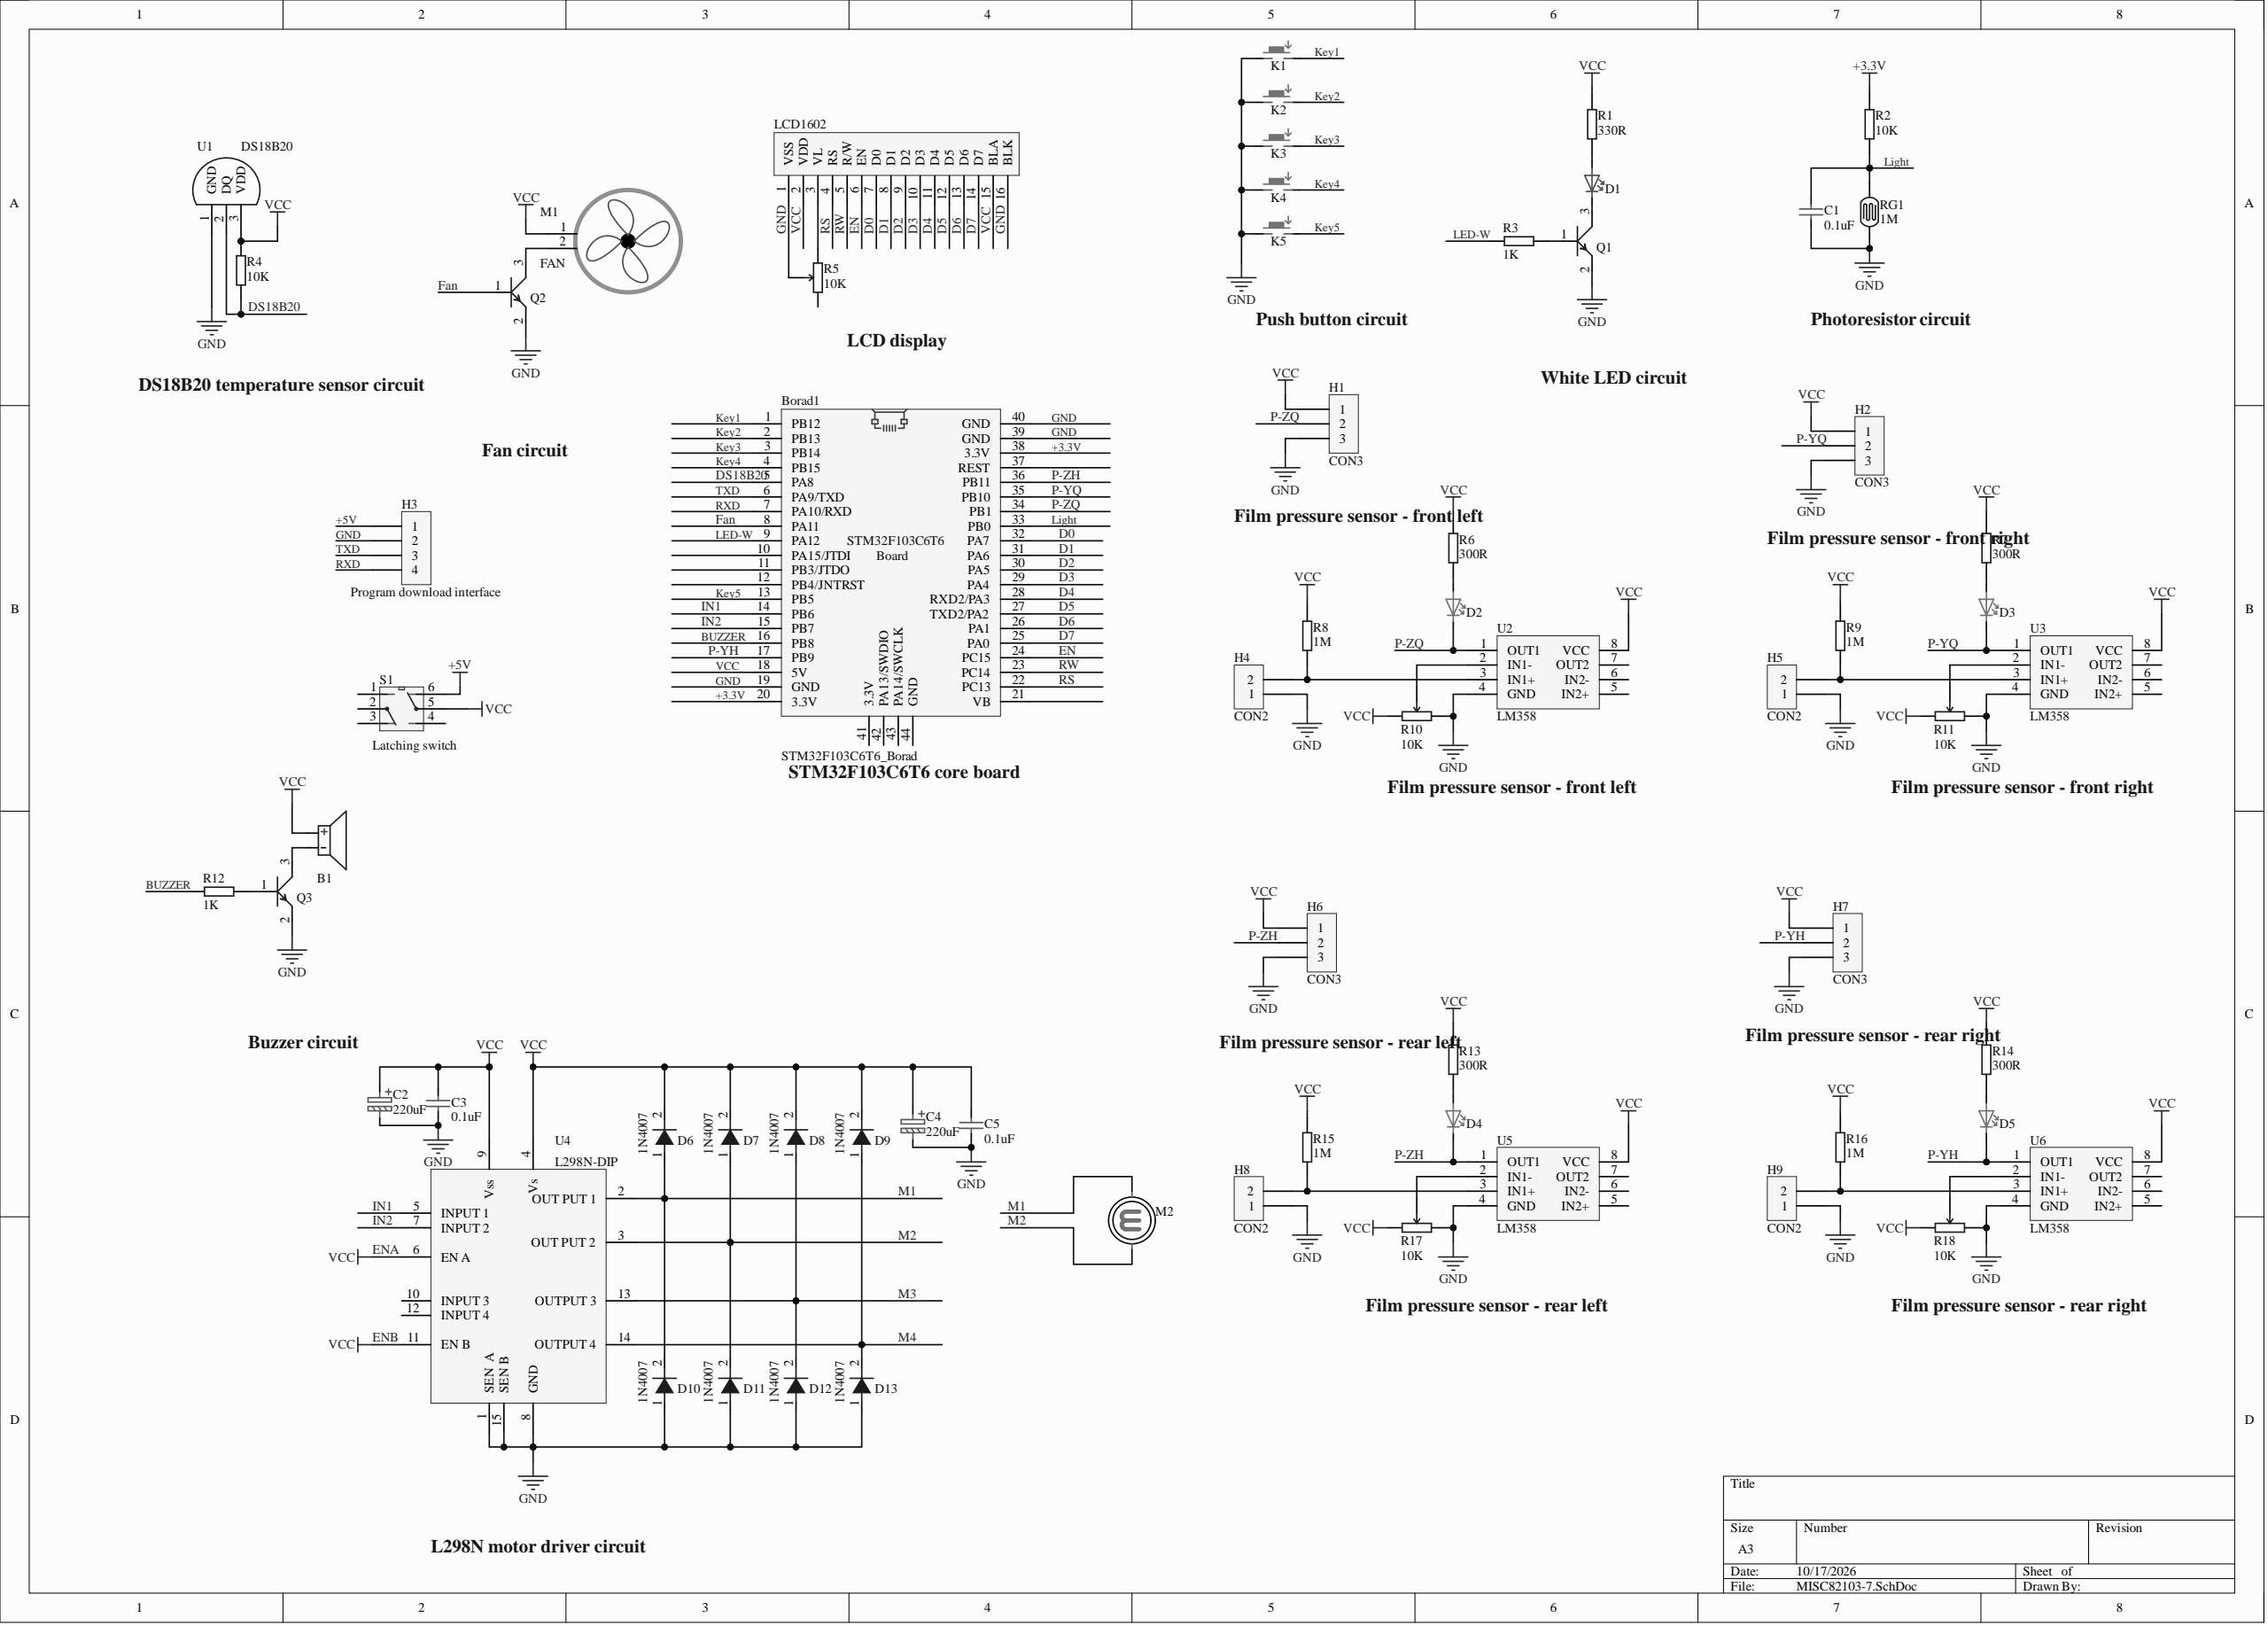Circuit board | Altium Designer | 66 parts | 56 nets
Bill of materials:
Comment,Description,Designator,Footprint,LibRef,Quantity
"Buzzer","Buzzer","B1","BUZZER","Buzzer","1"
"STM32F103C6T6_Borad","Core board (purchased online)","Borad1","STM32F103C8T6_买的","STM32F103C6T6_Borad","1"
"0.1uF","Non-polar capacitor","C1, C3, C5","CAP - 2.54mm","CAP","3"
"220uF","Polar capacitor","C2, C4","CAPe - 3.5MM","CAP-E","2"
"LED","LED","D1, D2, D3, D4, D5","LED-3MM","LED-RED, LED-GREEN","5"
"1N4007","Rectifier diode / single-direction diode","D6, D7, D8, D9, D10, D11, D12, D13","DIODE - 15.24mm","Diode","8"
"CON3","Pin header / terminal block / connector","H1, H2, H6, H7","CON3","CON3","4"
"Program download interface","Pin header / terminal block / connector","H3","CON4","CON4","1"
"CON2","Pin header / terminal block / connector","H4, H5, H8, H9","CON2","CON2","4"
"Key","Push button","K1, K2, K3, K4, K5","Buttom","Key","5"
"LCD1602","","LCD1","LCD1602","LCD1602","1"
"FAN","Small fan","M1","CON2","FAN","1"
"MOTTOR","DC motor","M2","CON2","MOTTOR","1"
"NPN","NPN transistor","Q1, Q2, Q3","NPN & PNP","NPN","3"
"330R","Resistor","R1","Resistor-7.62mm","Res","1"
"10K","Resistor","R2, R4","Resistor-7.62mm","Res","2"
"1K","Resistor","R3, R12","Resistor-7.62mm","Res","2"
"10K","Adjustable resistor","R5, R10, R11, R17, R18","Res_Variable-DIP","Res_Variable","5"
"300R","Resistor","R6, R7, R13, R14","Resistor-7.62mm","Res","4"
"1M","Resistor","R8, R9, R15, R16","Resistor-7.62mm","Res","4"
"1M","Photoresistor","RG1","RG","RG","1"
"Latching switch","8*8 power switch / latching switch","S1","Switch","Switch","1"
"DS18B20","Temperature sensor","U1","DS18B20","DS18B20","1"
"LM358","Dual operational amplifier","U2, U3, U5, U6","DIP8","LM358","4"
"L298N-DIP","Dual H-bridge driver IC","U4","L298N","L298N-DIP","1"
Netlist (Protel format):
[
B1
BUZZER
Buzzer



]
[
Borad1
STM32F103C8T6_买的
STM32F103C6T6_Borad



]
[
C1
CAP - 2.54mm
0.1uF



]
[
C2
CAPe - 3.5MM
220uF



]
[
C3
CAP - 2.54mm
0.1uF



]
[
C4
CAPe - 3.5MM
220uF



]
[
C5
CAP - 2.54mm
0.1uF



]
[
D1
LED-3MM
LED



]
[
D2
LED-3MM
LED



]
[
D3
LED-3MM
LED



]
[
D4
LED-3MM
LED



]
[
D5
LED-3MM
LED



]
[
D6
DIODE - 15.24mm
1N4007



]
[
D7
DIODE - 15.24mm
1N4007



]
[
D8
DIODE - 15.24mm
1N4007



]
[
D9
DIODE - 15.24mm
1N4007



]
[
D10
DIODE - 15.24mm
1N4007



]
[
D11
DIODE - 15.24mm
1N4007



]
[
D12
DIODE - 15.24mm
1N4007



]
[
D13
DIODE - 15.24mm
1N4007



]
[
H1
CON3
CON3



]
[
H2
CON3
CON3



]
[
H3
CON4
Program download interface



]
[
H4
CON2
CON2



]
[
H5
CON2
CON2



]
[
H6
CON3
CON3



]
[
H7
CON3
CON3



]
[
H8
CON2
CON2



]
[
H9
CON2
CON2



]
[
K1
Buttom
Key



]
[
K2
Buttom
Key



]
[
K3
Buttom
Key



]
[
K4
Buttom
Key



]
[
K5
Buttom
Key



]
[
LCD1
LCD1602
LCD1602



]
[
M1
CON2
FAN



]
[
M2
CON2
MOTTOR



]
[
Q1
NPN & PNP
NPN



]
[
Q2
NPN & PNP
NPN



]
[
Q3
NPN & PNP
NPN



]
[
R1
Resistor-7.62mm
330R



]
[
R2
Resistor-7.62mm
10K



]
[
R3
Resistor-7.62mm
1K



]
[
R4
Resistor-7.62mm
10K



]
[
R5
Res_Variable-DIP
10K



]
[
R6
Resistor-7.62mm
300R



]
[
R7
Resistor-7.62mm
300R



]
[
R8
Resistor-7.62mm
1M



]
[
R9
Resistor-7.62mm
1M



]
[
R10
Res_Variable-DIP
10K



]
[
R11
Res_Variable-DIP
10K



]
[
R12
Resistor-7.62mm
1K



]
[
R13
Resistor-7.62mm
300R



]
[
R14
Resistor-7.62mm
300R



]
[
R15
Resistor-7.62mm
1M



]
[
R16
Resistor-7.62mm
1M



]
[
R17
Res_Variable-DIP
10K



]
[
R18
Res_Variable-DIP
10K



]
[
RG1
RG
1M



]
[
S1
Switch
Latching switch



]
[
U1
DS18B20
DS18B20



]
[
U2
DIP8
LM358



]
[
U3
DIP8
LM358



]
[
U4
L298N
L298N-DIP



]
[
U5
DIP8
LM358



]
[
U6
DIP8
LM358



]
(
TXD
Borad1-6
H3-3
)
(
RXD
Borad1-7
H3-4
)
(
RW
Borad1-23
LCD1-5
)
(
RS
Borad1-22
LCD1-4
)
(
P-ZQ
Borad1-34
D2-1
H1-2
U2-1
)
(
P-ZH
Borad1-36
D4-1
H6-2
U5-1
)
(
P-YQ
Borad1-35
D3-1
H2-2
U3-1
)
(
P-YH
Borad1-17
D5-1
H7-2
U6-1
)
(
NetR18_2
R18-2
U6-2
)
(
NetR17_2
R17-2
U5-2
)
(
NetR11_2
R11-2
U3-2
)
(
NetR10_2
R10-2
U2-2
)
(
NetQ3_1
Q3-1
R12-2
)
(
NetQ1_1
Q1-1
R3-1
)
(
NetM1_2
M1-2
Q2-3
)
(
NetLCD1_3
LCD1-3
R5-1
)
(
NetH9_2
H9-2
R16-1
U6-3
)
(
NetH8_2
H8-2
R15-1
U5-3
)
(
NetH5_2
H5-2
R9-1
U3-3
)
(
NetH4_2
H4-2
R8-1
U2-3
)
(
NetD5_2
D5-2
R14-1
)
(
NetD4_2
D4-2
R13-1
)
(
NetD3_2
D3-2
R7-1
)
(
NetD2_2
D2-2
R6-1
)
(
NetD1_2
D1-2
R1-1
)
(
NetD1_1
D1-1
Q1-3
)
(
NetB1_2
B1-2
Q3-3
)
(
M4
D9-1
D13-2
U4-14
)
(
M3
D8-1
D12-2
U4-13
)
(
M2
D7-1
D11-2
M2-1
U4-3
)
(
M1
D6-1
D10-2
M2-2
U4-2
)
(
Light
Borad1-33
C1-2
R2-1
RG1-2
)
(
LED-W
Borad1-9
R3-2
)
(
Key5
Borad1-13
K5-2
)
(
Key4
Borad1-4
K4-2
)
(
Key3
Borad1-3
K3-2
)
(
Key2
Borad1-2
K2-2
)
(
Key1
Borad1-1
K1-2
)
(
IN2
Borad1-15
U4-7
)
(
IN1
Borad1-14
U4-5
)
(
GND
Borad1-19
Borad1-39
Borad1-40
C1-1
C2-2
C3-1
C4-2
C5-1
D10-1
D11-1
D12-1
D13-1
H1-3
H2-3
H3-2
H4-1
H5-1
H6-3
H7-3
H8-1
H9-1
K1-1
K2-1
K3-1
K4-1
K5-1
LCD1-1
LCD1-16
Q1-2
Q2-2
Q3-2
R5-2
R10-1
R11-1
R17-1
R18-1
RG1-1
U1-1
U2-4
U3-4
U4-1
U4-8
U4-15
U5-4
U6-4
)
(
Fan
Borad1-8
Q2-1
)
(
ENA
B1-1
Borad1-18
C2-1
C3-2
C4-1
C5-2
D6-2
D7-2
D8-2
D9-2
H1-1
H2-1
H6-1
H7-1
LCD1-2
LCD1-15
M1-1
R1-2
R4-1
R6-2
R7-2
R8-2
R9-2
R10-3
R11-3
R13-2
R14-2
R15-2
R16-2
R17-3
R18-3
S1-5
U1-3
U2-8
U3-8
U4-4
U4-6
U4-9
U4-11
U5-8
U6-8
)
(
EN
Borad1-24
LCD1-6
)
(
DS18B20
Borad1-5
R4-2
U1-2
)
(
D7
Borad1-25
LCD1-14
)
(
D6
Borad1-26
LCD1-13
)
(
D5
Borad1-27
LCD1-12
)
(
D4
Borad1-28
LCD1-11
)
(
D3
Borad1-29
LCD1-10
)
(
D2
Borad1-30
LCD1-9
)
(
D1
Borad1-31
LCD1-8
)
(
D0
Borad1-32
LCD1-7
)
(
BUZZER
Borad1-16
R12-1
)
(
+5V
H3-1
S1-6
)
(
+3.3V
Borad1-20
Borad1-38
R2-2
)